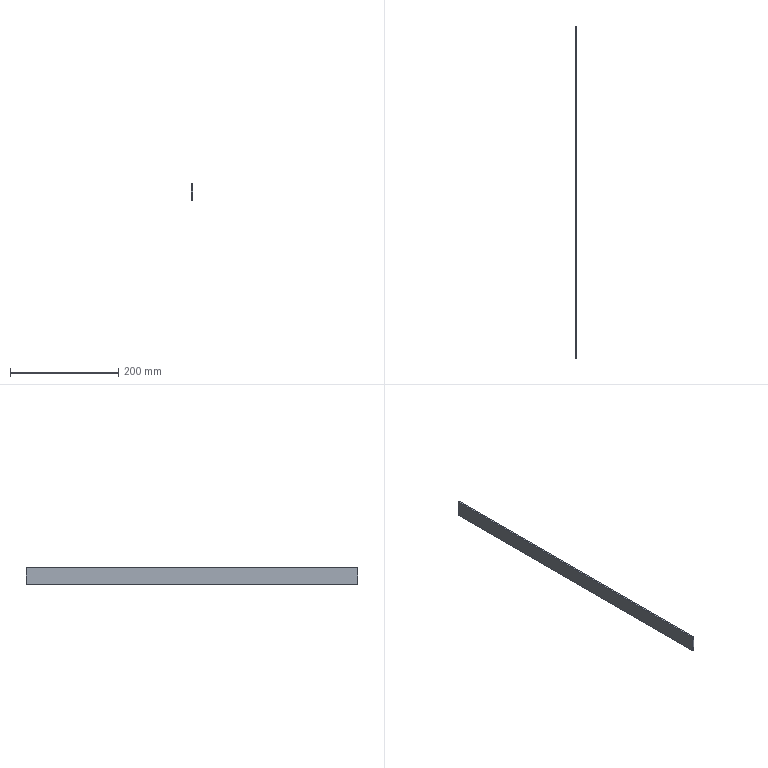Part | SolidWorks | 1 solid | 6 faces | box 3 x 612 x 30 mm | volume 55080 mm3 | plane 6
STEP:
#1=CARTESIAN_POINT('',(0.,306.,15.));
#2=VERTEX_POINT('',#1);
#3=CARTESIAN_POINT('',(0.,-306.,15.));
#4=VERTEX_POINT('',#3);
#5=CARTESIAN_POINT('',(0.,-306.,15.));
#6=DIRECTION('',(0.,-1.,0.));
#7=VECTOR('',#6,1000.);
#8=LINE('',#5,#7);
#9=EDGE_CURVE('',#2,#4,#8,.T.);
#10=ORIENTED_EDGE('',*,*,#9,.F.);
#11=CARTESIAN_POINT('',(-3.,306.,15.));
#12=VERTEX_POINT('',#11);
#13=CARTESIAN_POINT('',(-3.,306.,15.));
#14=DIRECTION('',(1.,0.,0.));
#15=VECTOR('',#14,1000.);
#16=LINE('',#13,#15);
#17=EDGE_CURVE('',#12,#2,#16,.T.);
#18=ORIENTED_EDGE('',*,*,#17,.F.);
#19=CARTESIAN_POINT('',(-3.,-306.,15.));
#20=VERTEX_POINT('',#19);
#21=CARTESIAN_POINT('',(-3.,-306.,15.));
#22=DIRECTION('',(0.,-1.,0.));
#23=VECTOR('',#22,1000.);
#24=LINE('',#21,#23);
#25=EDGE_CURVE('',#12,#20,#24,.T.);
#26=ORIENTED_EDGE('',*,*,#25,.T.);
#27=CARTESIAN_POINT('',(-3.,-306.,15.));
#28=DIRECTION('',(1.,0.,0.));
#29=VECTOR('',#28,1000.);
#30=LINE('',#27,#29);
#31=EDGE_CURVE('',#20,#4,#30,.T.);
#32=ORIENTED_EDGE('',*,*,#31,.T.);
#33=EDGE_LOOP('',(#10,#18,#26,#32));
#34=FACE_OUTER_BOUND('',#33,.T.);
#35=CARTESIAN_POINT('',(-3.,-306.,15.));
#36=DIRECTION('',(0.,0.,1.));
#37=DIRECTION('',(1.,0.,0.));
#38=AXIS2_PLACEMENT_3D('',#35,#36,#37);
#39=PLANE('',#38);
#40=ADVANCED_FACE('',(#34),#39,.T.);
#41=CARTESIAN_POINT('',(0.,306.,-15.));
#42=VERTEX_POINT('',#41);
#43=CARTESIAN_POINT('',(0.,306.,-15.));
#44=DIRECTION('',(0.,0.,1.));
#45=VECTOR('',#44,1000.);
#46=LINE('',#43,#45);
#47=EDGE_CURVE('',#42,#2,#46,.T.);
#48=ORIENTED_EDGE('',*,*,#47,.F.);
#49=CARTESIAN_POINT('',(-3.,306.,-15.));
#50=VERTEX_POINT('',#49);
#51=CARTESIAN_POINT('',(-3.,306.,-15.));
#52=DIRECTION('',(1.,0.,0.));
#53=VECTOR('',#52,1000.);
#54=LINE('',#51,#53);
#55=EDGE_CURVE('',#50,#42,#54,.T.);
#56=ORIENTED_EDGE('',*,*,#55,.F.);
#57=CARTESIAN_POINT('',(-3.,306.,-15.));
#58=DIRECTION('',(0.,0.,1.));
#59=VECTOR('',#58,1000.);
#60=LINE('',#57,#59);
#61=EDGE_CURVE('',#50,#12,#60,.T.);
#62=ORIENTED_EDGE('',*,*,#61,.T.);
#63=ORIENTED_EDGE('',*,*,#17,.T.);
#64=EDGE_LOOP('',(#48,#56,#62,#63));
#65=FACE_OUTER_BOUND('',#64,.T.);
#66=CARTESIAN_POINT('',(-3.,306.,-15.));
#67=DIRECTION('',(0.,1.,0.));
#68=DIRECTION('',(0.,0.,1.));
#69=AXIS2_PLACEMENT_3D('',#66,#67,#68);
#70=PLANE('',#69);
#71=ADVANCED_FACE('',(#65),#70,.T.);
#72=CARTESIAN_POINT('',(0.,-306.,-15.));
#73=VERTEX_POINT('',#72);
#74=CARTESIAN_POINT('',(0.,-306.,-15.));
#75=DIRECTION('',(0.,1.,0.));
#76=VECTOR('',#75,1000.);
#77=LINE('',#74,#76);
#78=EDGE_CURVE('',#73,#42,#77,.T.);
#79=ORIENTED_EDGE('',*,*,#78,.F.);
#80=CARTESIAN_POINT('',(-3.,-306.,-15.));
#81=VERTEX_POINT('',#80);
#82=CARTESIAN_POINT('',(-3.,-306.,-15.));
#83=DIRECTION('',(1.,0.,0.));
#84=VECTOR('',#83,1000.);
#85=LINE('',#82,#84);
#86=EDGE_CURVE('',#81,#73,#85,.T.);
#87=ORIENTED_EDGE('',*,*,#86,.F.);
#88=CARTESIAN_POINT('',(-3.,-306.,-15.));
#89=DIRECTION('',(0.,1.,0.));
#90=VECTOR('',#89,1000.);
#91=LINE('',#88,#90);
#92=EDGE_CURVE('',#81,#50,#91,.T.);
#93=ORIENTED_EDGE('',*,*,#92,.T.);
#94=ORIENTED_EDGE('',*,*,#55,.T.);
#95=EDGE_LOOP('',(#79,#87,#93,#94));
#96=FACE_OUTER_BOUND('',#95,.T.);
#97=CARTESIAN_POINT('',(-3.,-306.,-15.));
#98=DIRECTION('',(0.,0.,-1.));
#99=DIRECTION('',(-1.,0.,0.));
#100=AXIS2_PLACEMENT_3D('',#97,#98,#99);
#101=PLANE('',#100);
#102=ADVANCED_FACE('',(#96),#101,.T.);
#103=CARTESIAN_POINT('',(0.,-306.,-15.));
#104=DIRECTION('',(0.,0.,-1.));
#105=VECTOR('',#104,1000.);
#106=LINE('',#103,#105);
#107=EDGE_CURVE('',#4,#73,#106,.T.);
#108=ORIENTED_EDGE('',*,*,#107,.F.);
#109=ORIENTED_EDGE('',*,*,#31,.F.);
#110=CARTESIAN_POINT('',(-3.,-306.,-15.));
#111=DIRECTION('',(0.,0.,-1.));
#112=VECTOR('',#111,1000.);
#113=LINE('',#110,#112);
#114=EDGE_CURVE('',#20,#81,#113,.T.);
#115=ORIENTED_EDGE('',*,*,#114,.T.);
#116=ORIENTED_EDGE('',*,*,#86,.T.);
#117=EDGE_LOOP('',(#108,#109,#115,#116));
#118=FACE_OUTER_BOUND('',#117,.T.);
#119=CARTESIAN_POINT('',(-3.,-306.,-15.));
#120=DIRECTION('',(0.,-1.,0.));
#121=DIRECTION('',(0.,0.,-1.));
#122=AXIS2_PLACEMENT_3D('',#119,#120,#121);
#123=PLANE('',#122);
#124=ADVANCED_FACE('',(#118),#123,.T.);
#125=ORIENTED_EDGE('',*,*,#25,.F.);
#126=ORIENTED_EDGE('',*,*,#61,.F.);
#127=ORIENTED_EDGE('',*,*,#92,.F.);
#128=ORIENTED_EDGE('',*,*,#114,.F.);
#129=EDGE_LOOP('',(#125,#126,#127,#128));
#130=FACE_OUTER_BOUND('',#129,.T.);
#131=CARTESIAN_POINT('',(-3.,0.,0.));
#132=DIRECTION('',(1.,0.,0.));
#133=DIRECTION('',(0.,0.,-1.));
#134=AXIS2_PLACEMENT_3D('',#131,#132,#133);
#135=PLANE('',#134);
#136=ADVANCED_FACE('',(#130),#135,.F.);
#137=ORIENTED_EDGE('',*,*,#9,.T.);
#138=ORIENTED_EDGE('',*,*,#107,.T.);
#139=ORIENTED_EDGE('',*,*,#78,.T.);
#140=ORIENTED_EDGE('',*,*,#47,.T.);
#141=EDGE_LOOP('',(#137,#138,#139,#140));
#142=FACE_OUTER_BOUND('',#141,.T.);
#143=CARTESIAN_POINT('',(0.,0.,0.));
#144=DIRECTION('',(1.,0.,0.));
#145=DIRECTION('',(0.,0.,-1.));
#146=AXIS2_PLACEMENT_3D('',#143,#144,#145);
#147=PLANE('',#146);
#148=ADVANCED_FACE('',(#142),#147,.T.);
#149=CLOSED_SHELL('',(#40,#71,#102,#124,#136,#148));
#150=MANIFOLD_SOLID_BREP('',#149);
#151=CARTESIAN_POINT('',(0.,0.,0.));
#152=DIRECTION('',(0.,0.,1.));
#153=DIRECTION('',(1.,0.,0.));
#154=AXIS2_PLACEMENT_3D('',#151,#152,#153);
#155=(LENGTH_UNIT()NAMED_UNIT(*)SI_UNIT(.MILLI.,.METRE.));
#156=UNCERTAINTY_MEASURE_WITH_UNIT(LENGTH_MEASURE(0.00001),#155,'','');
#157=(NAMED_UNIT(*)PLANE_ANGLE_UNIT()SI_UNIT($,.RADIAN.));
#158=(NAMED_UNIT(*)SI_UNIT($,.STERADIAN.)SOLID_ANGLE_UNIT());
#159=(GEOMETRIC_REPRESENTATION_CONTEXT(3)GLOBAL_UNCERTAINTY_ASSIGNED_CONTEXT((#156))GLOBAL_UNIT_ASSIGNED_CONTEXT((#155,#157,#158))REPRESENTATION_CONTEXT('',''));
#160=ADVANCED_BREP_SHAPE_REPRESENTATION('',(#150,#154),#159);